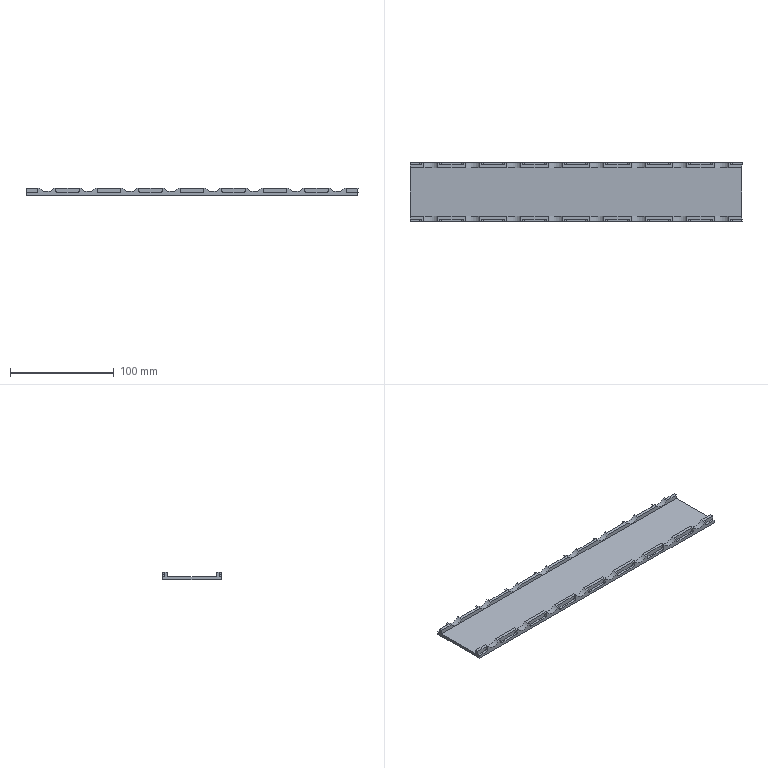Part | 1 solid | 142 faces | volume 61480 mm3 | plane 94 | cylinder 48 | commonest cylinder face diameters 4 x32 18.4 x16